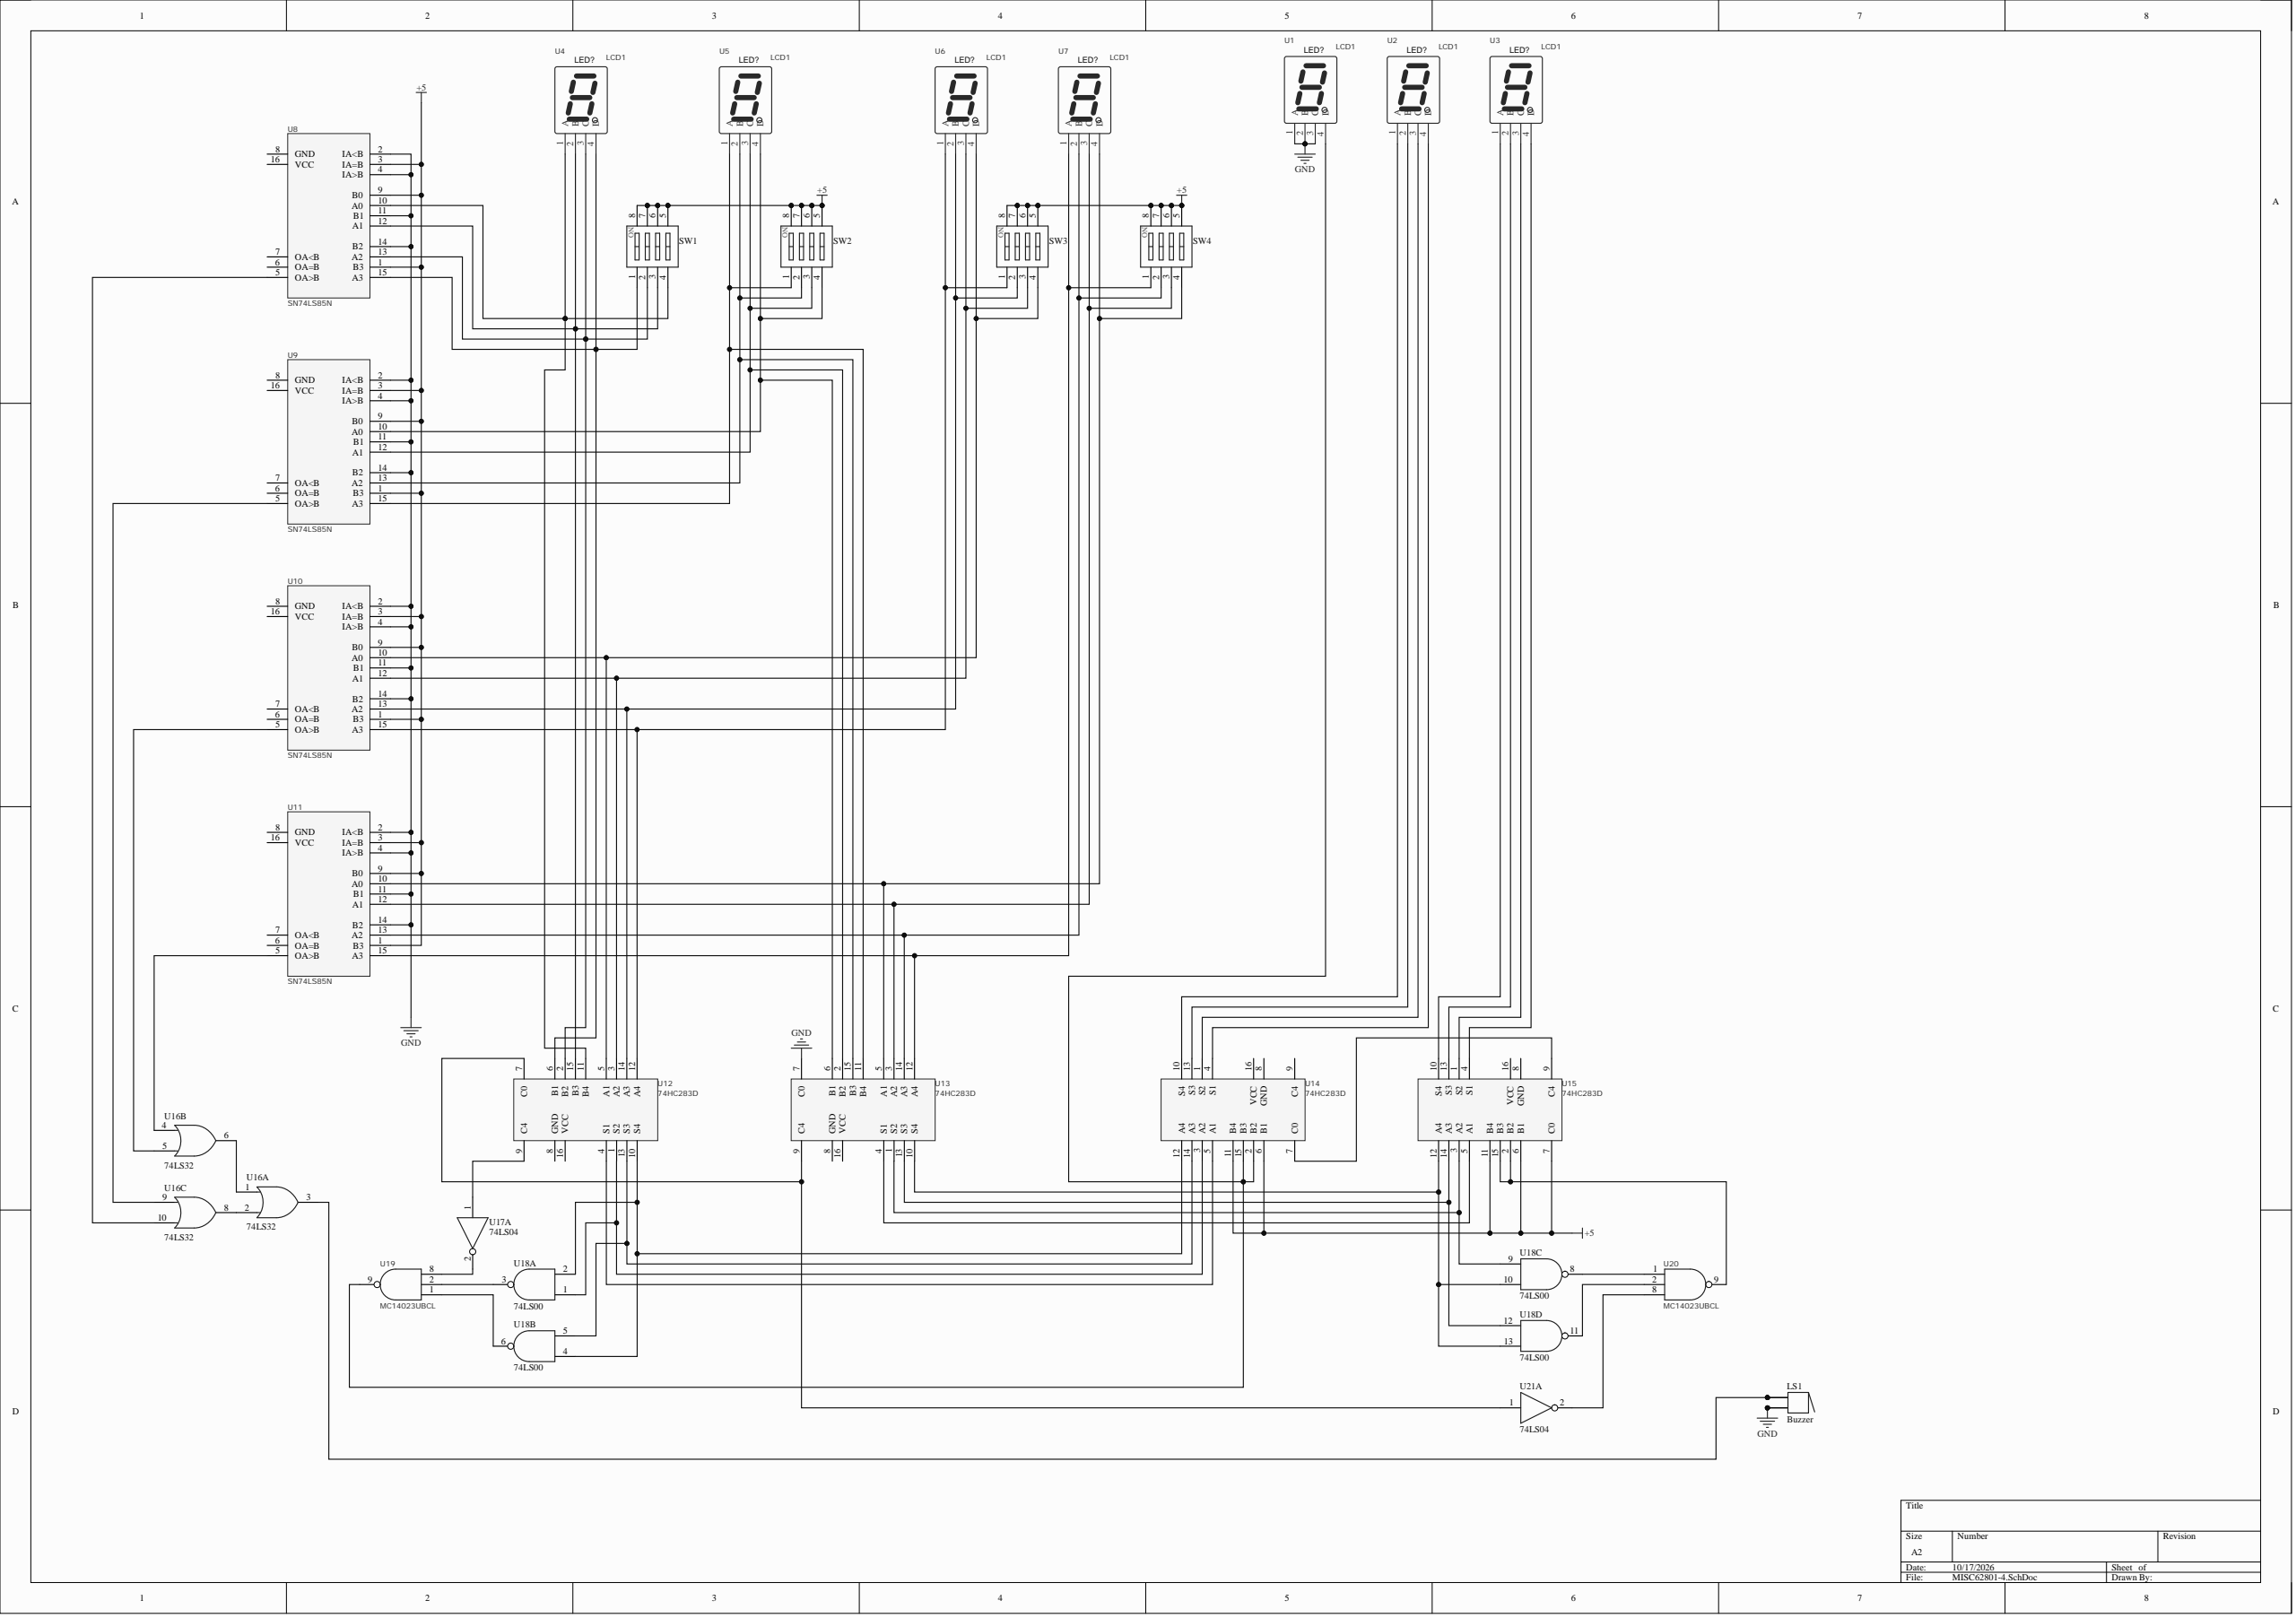Circuit board | Altium Designer | 26 parts | 52 nets
Bill of materials:
Comment,Description,Designator,Footprint,LibRef,Quantity
"Buzzer","Magnetic Transducer Buzzer","LS1","ABSM-1574","Buzzer","1"
"SW-4P","4-way coded switch","SW1, SW2, SW3, SW4","CSW DIP-4P","SW-4P","4"
"LCD1","","U1, U2, U3, U4, U5, U6, U7","DCD-HEX","LCD1","7"
"SN74LS85N","","U8, U9, U10, U11","DIP16","SN74LS85N","4"
"74HC283D","","U12, U13, U14, U15","DIP16","HD74HC283RP","4"
"74LS32","Quad 2-input OR gate","U16","DIP14","74LS32","1"
"74LS04","Hex inverter","U17, U21","DIP14","74LS04","2"
"74LS00","Quad 2-input NAND gate","U18","DIP14","74LS00","1"
"MC14023UBCL","","U19, U20","DIP14","MC14023UBCL","2"
Netlist (Protel format):
[
LS1
ABSM-1574
Buzzer



]
[
SW1
CSW DIP-4P
SW-4P



]
[
SW2
CSW DIP-4P
SW-4P



]
[
SW3
CSW DIP-4P
SW-4P



]
[
SW4
CSW DIP-4P
SW-4P



]
[
U1
DCD-HEX
LCD1



]
[
U2
DCD-HEX
LCD1



]
[
U3
DCD-HEX
LCD1



]
[
U4
DCD-HEX
LCD1



]
[
U5
DCD-HEX
LCD1



]
[
U6
DCD-HEX
LCD1



]
[
U7
DCD-HEX
LCD1



]
[
U8
DIP16
SN74LS85N



]
[
U9
DIP16
SN74LS85N



]
[
U10
DIP16
SN74LS85N



]
[
U11
DIP16
SN74LS85N



]
[
U12
DIP16
74HC283D



]
[
U13
DIP16
74HC283D



]
[
U14
DIP16
74HC283D



]
[
U15
DIP16
74HC283D



]
[
U16
DIP14
74LS32



]
[
U17
DIP14
74LS04



]
[
U18
DIP14
74LS00



]
[
U19
DIP14
MC14023UBCL



]
[
U20
DIP14
MC14023UBCL



]
[
U21
DIP14
74LS04



]
(
NetU20_8
U20-8
U21-2
)
(
NetU18_11
U18-11
U20-2
)
(
NetU18_8
U18-8
U20-1
)
(
NetU18_6
U18-6
U19-1
)
(
NetU18_3
U18-3
U19-2
)
(
NetU17_2
U17-2
U19-8
)
(
NetU16_2
U16-2
U16-8
)
(
NetU16_1
U16-1
U16-6
)
(
NetU15_12
U15-12
U18-10
U18-13
)
(
NetU15_2
U15-2
U15-15
U20-9
)
(
NetU14_7
U14-7
U15-9
)
(
NetU14_3
U14-3
U18-1
)
(
NetU13_13
U13-13
U15-14
U18-12
)
(
NetU13_4
U13-4
U15-5
)
(
NetU13_1
U13-1
U15-3
U18-9
)
(
NetU12_13
U12-13
U14-14
U18-5
)
(
NetU12_10
U12-10
U14-12
U18-2
U18-4
)
(
NetU12_9
U12-9
U17-1
)
(
NetU12_7
U12-7
U13-9
U21-1
)
(
NetU12_4
U12-4
U14-5
)
(
NetU11_5
U11-5
U16-4
)
(
NetU10_5
U10-5
U16-5
)
(
NetU9_5
U9-5
U16-9
)
(
NetU8_5
U8-5
U16-10
)
(
NetU3_4
U3-4
U15-4
)
(
NetU3_3
U3-3
U15-1
)
(
NetU3_2
U3-2
U15-13
)
(
NetU3_1
U3-1
U15-10
)
(
NetU2_4
U2-4
U14-4
)
(
NetU2_3
U2-3
U14-1
)
(
NetU2_2
U2-2
U14-13
)
(
NetU2_1
U2-1
U14-10
)
(
NetU1_4
U1-4
U14-2
U14-15
U19-9
)
(
NetSW4_4
SW4-4
U7-4
U11-10
U13-5
)
(
NetSW4_3
SW4-3
U7-3
U11-12
U13-3
)
(
NetSW4_2
SW4-2
U7-2
U11-13
U13-14
)
(
NetSW4_1
SW4-1
U7-1
U11-15
U13-12
)
(
NetSW3_4
SW3-4
U6-4
U10-10
U12-5
)
(
NetSW3_3
SW3-3
U6-3
U10-12
U12-3
)
(
NetSW3_2
SW3-2
U6-2
U10-13
U12-14
)
(
NetSW3_1
SW3-1
U6-1
U10-15
U12-12
)
(
NetSW2_4
SW2-4
U5-4
U9-10
U13-6
)
(
NetSW2_3
SW2-3
U5-3
U9-12
U13-2
)
(
NetSW2_2
SW2-2
U5-2
U9-13
U13-15
)
(
NetSW2_1
SW2-1
U5-1
U9-15
U13-11
)
(
NetSW1_4
SW1-4
U4-1
U8-10
U12-11
)
(
NetSW1_3
SW1-3
U4-2
U8-12
U12-15
)
(
NetSW1_2
SW1-2
U4-3
U8-13
U12-2
)
(
NetSW1_1
SW1-1
U4-4
U8-15
U12-6
)
(
NetLS1_1
LS1-1
LS1-1A
U16-3
)
(
GND
LS1-2
LS1-2A
U1-1
U1-2
U1-3
U8-2
U8-4
U8-11
U8-14
U9-2
U9-4
U9-11
U9-14
U10-2
U10-4
U10-11
U10-14
U11-2
U11-4
U11-11
U11-14
U13-7
)
(
+5
SW1-5
SW1-6
SW1-7
SW1-8
SW2-5
SW2-6
SW2-7
SW2-8
SW3-5
SW3-6
SW3-7
SW3-8
SW4-5
SW4-6
SW4-7
SW4-8
U8-1
U8-3
U8-9
U9-1
U9-3
U9-9
U10-1
U10-3
U10-9
U11-1
U11-3
U11-9
U14-6
U14-11
U15-6
U15-7
U15-11
)